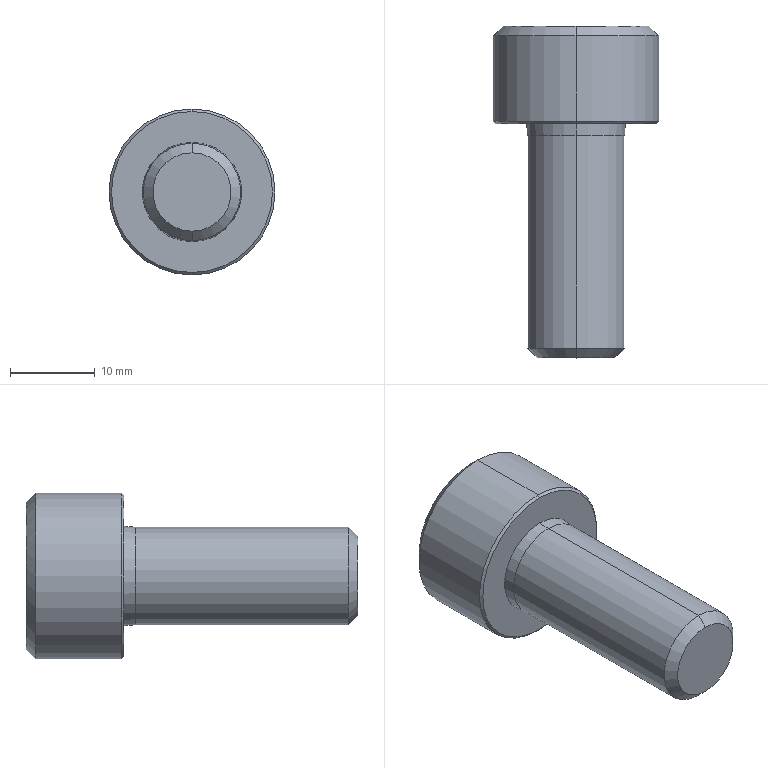Part | SolidWorks | features BaseBody 1 | 1 solid | 35 faces | box 19.615 x 39.231 x 19.615 mm | volume 5832 mm3 | cone 16 | plane 15 | cylinder 4 | commonest cylinder face diameters 11.538 x2 19.615 x2
STEP:
#1=CARTESIAN_POINT('',(-35.061,260.555,205.769));
#2=VERTEX_POINT('',#1);
#3=CARTESIAN_POINT('',(-35.061,260.555,194.231));
#4=VERTEX_POINT('',#3);
#5=CARTESIAN_POINT('',(-35.061,260.555,200.));
#6=DIRECTION('',(0.,1.,0.));
#7=DIRECTION('',(0.,0.,1.));
#8=AXIS2_PLACEMENT_3D('',#5,#6,#7);
#9=CIRCLE('',#8,5.769);
#10=EDGE_CURVE('',#2,#4,#9,.T.);
#11=ORIENTED_EDGE('',*,*,#10,.T.);
#12=CARTESIAN_POINT('',(-35.061,285.731,194.231));
#13=VERTEX_POINT('',#12);
#14=CARTESIAN_POINT('',(-35.061,259.423,194.231));
#15=DIRECTION('',(0.,1.,0.));
#16=VECTOR('',#15,1000.);
#17=LINE('',#14,#16);
#18=EDGE_CURVE('',#4,#13,#17,.T.);
#19=ORIENTED_EDGE('',*,*,#18,.T.);
#20=CARTESIAN_POINT('',(-35.061,285.731,205.769));
#21=VERTEX_POINT('',#20);
#22=CARTESIAN_POINT('',(-35.061,285.731,200.));
#23=DIRECTION('',(0.,-1.,0.));
#24=DIRECTION('',(0.,0.,1.));
#25=AXIS2_PLACEMENT_3D('',#22,#23,#24);
#26=CIRCLE('',#25,5.769);
#27=EDGE_CURVE('',#13,#21,#26,.T.);
#28=ORIENTED_EDGE('',*,*,#27,.T.);
#29=CARTESIAN_POINT('',(-35.061,259.423,205.769));
#30=DIRECTION('',(0.,1.,0.));
#31=VECTOR('',#30,1000.);
#32=LINE('',#29,#31);
#33=EDGE_CURVE('',#2,#21,#32,.T.);
#34=ORIENTED_EDGE('',*,*,#33,.F.);
#35=EDGE_LOOP('',(#11,#19,#28,#34));
#36=FACE_OUTER_BOUND('',#35,.T.);
#37=CARTESIAN_POINT('',(-35.061,259.423,200.));
#38=DIRECTION('',(0.,1.,0.));
#39=DIRECTION('',(0.,0.,1.));
#40=AXIS2_PLACEMENT_3D('',#37,#38,#39);
#41=CYLINDRICAL_SURFACE('',#40,5.769);
#42=ADVANCED_FACE('',(#36),#41,.T.);
#43=CARTESIAN_POINT('',(-35.061,259.423,204.637));
#44=VERTEX_POINT('',#43);
#45=CARTESIAN_POINT('',(-35.061,259.423,195.363));
#46=VERTEX_POINT('',#45);
#47=CARTESIAN_POINT('',(-35.061,259.423,200.));
#48=DIRECTION('',(0.,1.,0.));
#49=DIRECTION('',(0.,0.,1.));
#50=AXIS2_PLACEMENT_3D('',#47,#48,#49);
#51=CIRCLE('',#50,4.637);
#52=EDGE_CURVE('',#44,#46,#51,.T.);
#53=ORIENTED_EDGE('',*,*,#52,.T.);
#54=CARTESIAN_POINT('',(-35.061,260.555,194.231));
#55=DIRECTION('',(0.,0.7071,-0.7071));
#56=VECTOR('',#55,1000.);
#57=LINE('',#54,#56);
#58=EDGE_CURVE('',#46,#4,#57,.T.);
#59=ORIENTED_EDGE('',*,*,#58,.T.);
#60=ORIENTED_EDGE('',*,*,#10,.F.);
#61=CARTESIAN_POINT('',(-35.061,260.555,205.769));
#62=DIRECTION('',(0.,0.7071,0.7071));
#63=VECTOR('',#62,1000.);
#64=LINE('',#61,#63);
#65=EDGE_CURVE('',#44,#2,#64,.T.);
#66=ORIENTED_EDGE('',*,*,#65,.F.);
#67=EDGE_LOOP('',(#53,#59,#60,#66));
#68=FACE_OUTER_BOUND('',#67,.T.);
#69=CARTESIAN_POINT('',(-35.061,260.555,200.));
#70=DIRECTION('',(0.,1.,0.));
#71=DIRECTION('',(0.,0.,1.));
#72=AXIS2_PLACEMENT_3D('',#69,#70,#71);
#73=CONICAL_SURFACE('',#72,5.769,0.7854);
#74=ADVANCED_FACE('',(#68),#73,.T.);
#75=ORIENTED_EDGE('',*,*,#27,.F.);
#76=CARTESIAN_POINT('',(-35.061,287.115,194.115));
#77=VERTEX_POINT('',#76);
#78=CARTESIAN_POINT('',(-35.061,287.115,194.115));
#79=DIRECTION('',(0.,0.9965,-0.08305));
#80=VECTOR('',#79,1000.);
#81=LINE('',#78,#80);
#82=EDGE_CURVE('',#13,#77,#81,.T.);
#83=ORIENTED_EDGE('',*,*,#82,.T.);
#84=CARTESIAN_POINT('',(-35.061,287.115,205.885));
#85=VERTEX_POINT('',#84);
#86=CARTESIAN_POINT('',(-35.061,287.115,200.));
#87=DIRECTION('',(0.,-1.,0.));
#88=DIRECTION('',(0.,0.,1.));
#89=AXIS2_PLACEMENT_3D('',#86,#87,#88);
#90=CIRCLE('',#89,5.885);
#91=EDGE_CURVE('',#77,#85,#90,.T.);
#92=ORIENTED_EDGE('',*,*,#91,.T.);
#93=CARTESIAN_POINT('',(-35.061,287.115,205.885));
#94=DIRECTION('',(0.,0.9965,0.08305));
#95=VECTOR('',#94,1000.);
#96=LINE('',#93,#95);
#97=EDGE_CURVE('',#21,#85,#96,.T.);
#98=ORIENTED_EDGE('',*,*,#97,.F.);
#99=EDGE_LOOP('',(#75,#83,#92,#98));
#100=FACE_OUTER_BOUND('',#99,.T.);
#101=CARTESIAN_POINT('',(-35.061,287.115,200.));
#102=DIRECTION('',(0.,1.,0.));
#103=DIRECTION('',(0.,0.,1.));
#104=AXIS2_PLACEMENT_3D('',#101,#102,#103);
#105=CONICAL_SURFACE('',#104,5.885,0.08314);
#106=ADVANCED_FACE('',(#100),#105,.T.);
#107=CARTESIAN_POINT('',(-35.061,287.115,209.519));
#108=VERTEX_POINT('',#107);
#109=CARTESIAN_POINT('',(-35.061,287.115,190.481));
#110=VERTEX_POINT('',#109);
#111=CARTESIAN_POINT('',(-35.061,287.115,200.));
#112=DIRECTION('',(0.,1.,0.));
#113=DIRECTION('',(0.,0.,1.));
#114=AXIS2_PLACEMENT_3D('',#111,#112,#113);
#115=CIRCLE('',#114,9.519);
#116=EDGE_CURVE('',#108,#110,#115,.T.);
#117=ORIENTED_EDGE('',*,*,#116,.T.);
#118=CARTESIAN_POINT('',(-35.061,287.404,190.192));
#119=VERTEX_POINT('',#118);
#120=CARTESIAN_POINT('',(-35.061,287.404,190.192));
#121=DIRECTION('',(0.,0.7071,-0.7071));
#122=VECTOR('',#121,1000.);
#123=LINE('',#120,#122);
#124=EDGE_CURVE('',#110,#119,#123,.T.);
#125=ORIENTED_EDGE('',*,*,#124,.T.);
#126=CARTESIAN_POINT('',(-35.061,287.404,209.808));
#127=VERTEX_POINT('',#126);
#128=CARTESIAN_POINT('',(-35.061,287.404,200.));
#129=DIRECTION('',(0.,-1.,0.));
#130=DIRECTION('',(0.,0.,1.));
#131=AXIS2_PLACEMENT_3D('',#128,#129,#130);
#132=CIRCLE('',#131,9.808);
#133=EDGE_CURVE('',#119,#127,#132,.T.);
#134=ORIENTED_EDGE('',*,*,#133,.T.);
#135=CARTESIAN_POINT('',(-35.061,287.404,209.808));
#136=DIRECTION('',(0.,0.7071,0.7071));
#137=VECTOR('',#136,1000.);
#138=LINE('',#135,#137);
#139=EDGE_CURVE('',#108,#127,#138,.T.);
#140=ORIENTED_EDGE('',*,*,#139,.F.);
#141=EDGE_LOOP('',(#117,#125,#134,#140));
#142=FACE_OUTER_BOUND('',#141,.T.);
#143=CARTESIAN_POINT('',(-35.061,287.404,200.));
#144=DIRECTION('',(0.,1.,0.));
#145=DIRECTION('',(0.,0.,1.));
#146=AXIS2_PLACEMENT_3D('',#143,#144,#145);
#147=CONICAL_SURFACE('',#146,9.808,0.7854);
#148=ADVANCED_FACE('',(#142),#147,.T.);
#149=ORIENTED_EDGE('',*,*,#133,.F.);
#150=CARTESIAN_POINT('',(-35.061,297.5,190.192));
#151=VERTEX_POINT('',#150);
#152=CARTESIAN_POINT('',(-35.061,259.423,190.192));
#153=DIRECTION('',(0.,1.,0.));
#154=VECTOR('',#153,1000.);
#155=LINE('',#152,#154);
#156=EDGE_CURVE('',#119,#151,#155,.T.);
#157=ORIENTED_EDGE('',*,*,#156,.T.);
#158=CARTESIAN_POINT('',(-35.061,297.5,209.808));
#159=VERTEX_POINT('',#158);
#160=CARTESIAN_POINT('',(-35.061,297.5,200.));
#161=DIRECTION('',(0.,-1.,0.));
#162=DIRECTION('',(0.,0.,1.));
#163=AXIS2_PLACEMENT_3D('',#160,#161,#162);
#164=CIRCLE('',#163,9.808);
#165=EDGE_CURVE('',#151,#159,#164,.T.);
#166=ORIENTED_EDGE('',*,*,#165,.T.);
#167=CARTESIAN_POINT('',(-35.061,259.423,209.808));
#168=DIRECTION('',(0.,1.,0.));
#169=VECTOR('',#168,1000.);
#170=LINE('',#167,#169);
#171=EDGE_CURVE('',#127,#159,#170,.T.);
#172=ORIENTED_EDGE('',*,*,#171,.F.);
#173=EDGE_LOOP('',(#149,#157,#166,#172));
#174=FACE_OUTER_BOUND('',#173,.T.);
#175=CARTESIAN_POINT('',(-35.061,259.423,200.));
#176=DIRECTION('',(0.,1.,0.));
#177=DIRECTION('',(0.,0.,1.));
#178=AXIS2_PLACEMENT_3D('',#175,#176,#177);
#179=CYLINDRICAL_SURFACE('',#178,9.808);
#180=ADVANCED_FACE('',(#174),#179,.T.);
#181=CARTESIAN_POINT('',(-35.061,298.654,191.346));
#182=VERTEX_POINT('',#181);
#183=CARTESIAN_POINT('',(-35.061,298.654,208.654));
#184=VERTEX_POINT('',#183);
#185=CARTESIAN_POINT('',(-35.061,298.654,200.));
#186=DIRECTION('',(0.,-1.,0.));
#187=DIRECTION('',(0.,0.,-1.));
#188=AXIS2_PLACEMENT_3D('',#185,#186,#187);
#189=CIRCLE('',#188,8.654);
#190=EDGE_CURVE('',#182,#184,#189,.T.);
#191=ORIENTED_EDGE('',*,*,#190,.T.);
#192=CARTESIAN_POINT('',(-35.061,297.5,209.808));
#193=DIRECTION('',(0.,-0.7071,0.7071));
#194=VECTOR('',#193,1000.);
#195=LINE('',#192,#194);
#196=EDGE_CURVE('',#184,#159,#195,.T.);
#197=ORIENTED_EDGE('',*,*,#196,.T.);
#198=ORIENTED_EDGE('',*,*,#165,.F.);
#199=CARTESIAN_POINT('',(-35.061,297.5,190.192));
#200=DIRECTION('',(0.,-0.7071,-0.7071));
#201=VECTOR('',#200,1000.);
#202=LINE('',#199,#201);
#203=EDGE_CURVE('',#182,#151,#202,.T.);
#204=ORIENTED_EDGE('',*,*,#203,.F.);
#205=EDGE_LOOP('',(#191,#197,#198,#204));
#206=FACE_OUTER_BOUND('',#205,.T.);
#207=CARTESIAN_POINT('',(-35.061,297.5,200.));
#208=DIRECTION('',(0.,-1.,0.));
#209=DIRECTION('',(0.,0.,-1.));
#210=AXIS2_PLACEMENT_3D('',#207,#208,#209);
#211=CONICAL_SURFACE('',#210,9.808,0.7854);
#212=ADVANCED_FACE('',(#206),#211,.T.);
#213=CARTESIAN_POINT('',(-35.061,290.22,200.));
#214=VERTEX_POINT('',#213);
#215=CARTESIAN_POINT('',(-35.061,292.885,204.615));
#216=VERTEX_POINT('',#215);
#217=CARTESIAN_POINT('',(-35.061,292.885,204.615));
#218=DIRECTION('',(0.,0.5,0.866));
#219=VECTOR('',#218,1000.);
#220=LINE('',#217,#219);
#221=EDGE_CURVE('',#214,#216,#220,.T.);
#222=ORIENTED_EDGE('',*,*,#221,.F.);
#223=CARTESIAN_POINT('',(-35.061,292.885,195.385));
#224=VERTEX_POINT('',#223);
#225=CARTESIAN_POINT('',(-35.061,292.885,195.385));
#226=DIRECTION('',(0.,0.5,-0.866));
#227=VECTOR('',#226,1000.);
#228=LINE('',#225,#227);
#229=EDGE_CURVE('',#214,#224,#228,.T.);
#230=ORIENTED_EDGE('',*,*,#229,.T.);
#231=CARTESIAN_POINT('',(-37.369,292.885,196.003));
#232=VERTEX_POINT('',#231);
#233=CARTESIAN_POINT('',(-35.061,292.885,200.));
#234=DIRECTION('',(0.,-1.,0.));
#235=DIRECTION('',(0.,0.,1.));
#236=AXIS2_PLACEMENT_3D('',#233,#234,#235);
#237=CIRCLE('',#236,4.615);
#238=EDGE_CURVE('',#232,#224,#237,.T.);
#239=ORIENTED_EDGE('',*,*,#238,.F.);
#240=CARTESIAN_POINT('',(-39.677,292.885,200.));
#241=VERTEX_POINT('',#240);
#242=CARTESIAN_POINT('',(-35.061,292.885,200.));
#243=DIRECTION('',(0.,-1.,0.));
#244=DIRECTION('',(0.,0.,1.));
#245=AXIS2_PLACEMENT_3D('',#242,#243,#244);
#246=CIRCLE('',#245,4.615);
#247=EDGE_CURVE('',#241,#232,#246,.T.);
#248=ORIENTED_EDGE('',*,*,#247,.F.);
#249=CARTESIAN_POINT('',(-37.369,292.885,203.997));
#250=VERTEX_POINT('',#249);
#251=CARTESIAN_POINT('',(-35.061,292.885,200.));
#252=DIRECTION('',(0.,-1.,0.));
#253=DIRECTION('',(0.,0.,1.));
#254=AXIS2_PLACEMENT_3D('',#251,#252,#253);
#255=CIRCLE('',#254,4.615);
#256=EDGE_CURVE('',#250,#241,#255,.T.);
#257=ORIENTED_EDGE('',*,*,#256,.F.);
#258=CARTESIAN_POINT('',(-35.061,292.885,200.));
#259=DIRECTION('',(0.,-1.,0.));
#260=DIRECTION('',(0.,0.,1.));
#261=AXIS2_PLACEMENT_3D('',#258,#259,#260);
#262=CIRCLE('',#261,4.615);
#263=EDGE_CURVE('',#216,#250,#262,.T.);
#264=ORIENTED_EDGE('',*,*,#263,.F.);
#265=EDGE_LOOP('',(#222,#230,#239,#248,#257,#264));
#266=FACE_OUTER_BOUND('',#265,.T.);
#267=CARTESIAN_POINT('',(-35.061,292.885,200.));
#268=DIRECTION('',(0.,1.,0.));
#269=DIRECTION('',(0.,0.,1.));
#270=AXIS2_PLACEMENT_3D('',#267,#268,#269);
#271=CONICAL_SURFACE('',#270,4.615,1.047);
#272=ADVANCED_FACE('',(#266),#271,.F.);
#273=ORIENTED_EDGE('',*,*,#18,.F.);
#274=CARTESIAN_POINT('',(-35.061,260.555,200.));
#275=DIRECTION('',(0.,1.,0.));
#276=DIRECTION('',(0.,0.,1.));
#277=AXIS2_PLACEMENT_3D('',#274,#275,#276);
#278=CIRCLE('',#277,5.769);
#279=EDGE_CURVE('',#4,#2,#278,.T.);
#280=ORIENTED_EDGE('',*,*,#279,.T.);
#281=ORIENTED_EDGE('',*,*,#33,.T.);
#282=CARTESIAN_POINT('',(-35.061,285.731,200.));
#283=DIRECTION('',(0.,-1.,0.));
#284=DIRECTION('',(0.,0.,1.));
#285=AXIS2_PLACEMENT_3D('',#282,#283,#284);
#286=CIRCLE('',#285,5.769);
#287=EDGE_CURVE('',#21,#13,#286,.T.);
#288=ORIENTED_EDGE('',*,*,#287,.T.);
#289=EDGE_LOOP('',(#273,#280,#281,#288));
#290=FACE_OUTER_BOUND('',#289,.T.);
#291=CARTESIAN_POINT('',(-35.061,259.423,200.));
#292=DIRECTION('',(0.,1.,0.));
#293=DIRECTION('',(0.,0.,1.));
#294=AXIS2_PLACEMENT_3D('',#291,#292,#293);
#295=CYLINDRICAL_SURFACE('',#294,5.769);
#296=ADVANCED_FACE('',(#290),#295,.T.);
#297=ORIENTED_EDGE('',*,*,#58,.F.);
#298=CARTESIAN_POINT('',(-35.061,259.423,200.));
#299=DIRECTION('',(0.,1.,0.));
#300=DIRECTION('',(0.,0.,1.));
#301=AXIS2_PLACEMENT_3D('',#298,#299,#300);
#302=CIRCLE('',#301,4.637);
#303=EDGE_CURVE('',#46,#44,#302,.T.);
#304=ORIENTED_EDGE('',*,*,#303,.T.);
#305=ORIENTED_EDGE('',*,*,#65,.T.);
#306=ORIENTED_EDGE('',*,*,#279,.F.);
#307=EDGE_LOOP('',(#297,#304,#305,#306));
#308=FACE_OUTER_BOUND('',#307,.T.);
#309=CARTESIAN_POINT('',(-35.061,260.555,200.));
#310=DIRECTION('',(0.,1.,0.));
#311=DIRECTION('',(0.,0.,1.));
#312=AXIS2_PLACEMENT_3D('',#309,#310,#311);
#313=CONICAL_SURFACE('',#312,5.769,0.7854);
#314=ADVANCED_FACE('',(#308),#313,.T.);
#315=ORIENTED_EDGE('',*,*,#82,.F.);
#316=ORIENTED_EDGE('',*,*,#287,.F.);
#317=ORIENTED_EDGE('',*,*,#97,.T.);
#318=CARTESIAN_POINT('',(-35.061,287.115,200.));
#319=DIRECTION('',(0.,-1.,0.));
#320=DIRECTION('',(0.,0.,1.));
#321=AXIS2_PLACEMENT_3D('',#318,#319,#320);
#322=CIRCLE('',#321,5.885);
#323=EDGE_CURVE('',#85,#77,#322,.T.);
#324=ORIENTED_EDGE('',*,*,#323,.T.);
#325=EDGE_LOOP('',(#315,#316,#317,#324));
#326=FACE_OUTER_BOUND('',#325,.T.);
#327=CARTESIAN_POINT('',(-35.061,287.115,200.));
#328=DIRECTION('',(0.,1.,0.));
#329=DIRECTION('',(0.,0.,1.));
#330=AXIS2_PLACEMENT_3D('',#327,#328,#329);
#331=CONICAL_SURFACE('',#330,5.885,0.08314);
#332=ADVANCED_FACE('',(#326),#331,.T.);
#333=ORIENTED_EDGE('',*,*,#52,.F.);
#334=ORIENTED_EDGE('',*,*,#303,.F.);
#335=EDGE_LOOP('',(#333,#334));
#336=FACE_OUTER_BOUND('',#335,.T.);
#337=CARTESIAN_POINT('',(-39.698,259.423,200.));
#338=DIRECTION('',(0.,1.,0.));
#339=DIRECTION('',(0.,0.,1.));
#340=AXIS2_PLACEMENT_3D('',#337,#338,#339);
#341=PLANE('',#340);
#342=ADVANCED_FACE('',(#336),#341,.F.);
#343=ORIENTED_EDGE('',*,*,#323,.F.);
#344=ORIENTED_EDGE('',*,*,#91,.F.);
#345=EDGE_LOOP('',(#343,#344));
#346=FACE_BOUND('',#345,.T.);
#347=ORIENTED_EDGE('',*,*,#116,.F.);
#348=CARTESIAN_POINT('',(-35.061,287.115,200.));
#349=DIRECTION('',(0.,1.,0.));
#350=DIRECTION('',(0.,0.,1.));
#351=AXIS2_PLACEMENT_3D('',#348,#349,#350);
#352=CIRCLE('',#351,9.519);
#353=EDGE_CURVE('',#110,#108,#352,.T.);
#354=ORIENTED_EDGE('',*,*,#353,.F.);
#355=EDGE_LOOP('',(#347,#354));
#356=FACE_OUTER_BOUND('',#355,.T.);
#357=CARTESIAN_POINT('',(-44.58,287.115,200.));
#358=DIRECTION('',(0.,1.,0.));
#359=DIRECTION('',(0.,0.,1.));
#360=AXIS2_PLACEMENT_3D('',#357,#358,#359);
#361=PLANE('',#360);
#362=ADVANCED_FACE('',(#346,#356),#361,.F.);
#363=ORIENTED_EDGE('',*,*,#124,.F.);
#364=ORIENTED_EDGE('',*,*,#353,.T.);
#365=ORIENTED_EDGE('',*,*,#139,.T.);
#366=CARTESIAN_POINT('',(-35.061,287.404,200.));
#367=DIRECTION('',(0.,-1.,0.));
#368=DIRECTION('',(0.,0.,1.));
#369=AXIS2_PLACEMENT_3D('',#366,#367,#368);
#370=CIRCLE('',#369,9.808);
#371=EDGE_CURVE('',#127,#119,#370,.T.);
#372=ORIENTED_EDGE('',*,*,#371,.T.);
#373=EDGE_LOOP('',(#363,#364,#365,#372));
#374=FACE_OUTER_BOUND('',#373,.T.);
#375=CARTESIAN_POINT('',(-35.061,287.404,200.));
#376=DIRECTION('',(0.,1.,0.));
#377=DIRECTION('',(0.,0.,1.));
#378=AXIS2_PLACEMENT_3D('',#375,#376,#377);
#379=CONICAL_SURFACE('',#378,9.808,0.7854);
#380=ADVANCED_FACE('',(#374),#379,.T.);
#381=ORIENTED_EDGE('',*,*,#156,.F.);
#382=ORIENTED_EDGE('',*,*,#371,.F.);
#383=ORIENTED_EDGE('',*,*,#171,.T.);
#384=CARTESIAN_POINT('',(-35.061,297.5,200.));
#385=DIRECTION('',(0.,-1.,0.));
#386=DIRECTION('',(0.,0.,1.));
#387=AXIS2_PLACEMENT_3D('',#384,#385,#386);
#388=CIRCLE('',#387,9.808);
#389=EDGE_CURVE('',#159,#151,#388,.T.);
#390=ORIENTED_EDGE('',*,*,#389,.T.);
#391=EDGE_LOOP('',(#381,#382,#383,#390));
#392=FACE_OUTER_BOUND('',#391,.T.);
#393=CARTESIAN_POINT('',(-35.061,259.423,200.));
#394=DIRECTION('',(0.,1.,0.));
#395=DIRECTION('',(0.,0.,1.));
#396=AXIS2_PLACEMENT_3D('',#393,#394,#395);
#397=CYLINDRICAL_SURFACE('',#396,9.808);
#398=ADVANCED_FACE('',(#392),#397,.T.);
#399=ORIENTED_EDGE('',*,*,#196,.F.);
#400=CARTESIAN_POINT('',(-35.061,298.654,200.));
#401=DIRECTION('',(0.,-1.,0.));
#402=DIRECTION('',(0.,0.,-1.));
#403=AXIS2_PLACEMENT_3D('',#400,#401,#402);
#404=CIRCLE('',#403,8.654);
#405=EDGE_CURVE('',#184,#182,#404,.T.);
#406=ORIENTED_EDGE('',*,*,#405,.T.);
#407=ORIENTED_EDGE('',*,*,#203,.T.);
#408=ORIENTED_EDGE('',*,*,#389,.F.);
#409=EDGE_LOOP('',(#399,#406,#407,#408));
#410=FACE_OUTER_BOUND('',#409,.T.);
#411=CARTESIAN_POINT('',(-35.061,297.5,200.));
#412=DIRECTION('',(0.,-1.,0.));
#413=DIRECTION('',(0.,0.,-1.));
#414=AXIS2_PLACEMENT_3D('',#411,#412,#413);
#415=CONICAL_SURFACE('',#414,9.808,0.7854);
#416=ADVANCED_FACE('',(#410),#415,.T.);
#417=CARTESIAN_POINT('',(-30.446,298.654,197.335));
#418=VERTEX_POINT('',#417);
#419=CARTESIAN_POINT('',(-35.061,298.654,194.671));
#420=VERTEX_POINT('',#419);
#421=CARTESIAN_POINT('',(-35.061,298.654,200.));
#422=DIRECTION('',(0.,1.,0.));
#423=DIRECTION('',(0.,0.,1.));
#424=AXIS2_PLACEMENT_3D('',#421,#422,#423);
#425=CIRCLE('',#424,5.329);
#426=EDGE_CURVE('',#418,#420,#425,.T.);
#427=ORIENTED_EDGE('',*,*,#426,.F.);
#428=CARTESIAN_POINT('',(-30.446,298.654,202.665));
#429=VERTEX_POINT('',#428);
#430=CARTESIAN_POINT('',(-35.061,298.654,200.));
#431=DIRECTION('',(0.,1.,0.));
#432=DIRECTION('',(0.,0.,1.));
#433=AXIS2_PLACEMENT_3D('',#430,#431,#432);
#434=CIRCLE('',#433,5.329);
#435=EDGE_CURVE('',#429,#418,#434,.T.);
#436=ORIENTED_EDGE('',*,*,#435,.F.);
#437=CARTESIAN_POINT('',(-35.061,298.654,205.329));
#438=VERTEX_POINT('',#437);
#439=CARTESIAN_POINT('',(-35.061,298.654,200.));
#440=DIRECTION('',(0.,1.,0.));
#441=DIRECTION('',(0.,0.,1.));
#442=AXIS2_PLACEMENT_3D('',#439,#440,#441);
#443=CIRCLE('',#442,5.329);
#444=EDGE_CURVE('',#438,#429,#443,.T.);
#445=ORIENTED_EDGE('',*,*,#444,.F.);
#446=CARTESIAN_POINT('',(-39.677,298.654,202.665));
#447=VERTEX_POINT('',#446);
#448=CARTESIAN_POINT('',(-35.061,298.654,200.));
#449=DIRECTION('',(0.,1.,0.));
#450=DIRECTION('',(0.,0.,1.));
#451=AXIS2_PLACEMENT_3D('',#448,#449,#450);
#452=CIRCLE('',#451,5.329);
#453=EDGE_CURVE('',#447,#438,#452,.T.);
#454=ORIENTED_EDGE('',*,*,#453,.F.);
#455=CARTESIAN_POINT('',(-39.677,298.654,197.335));
#456=VERTEX_POINT('',#455);
#457=CARTESIAN_POINT('',(-35.061,298.654,200.));
#458=DIRECTION('',(0.,1.,0.));
#459=DIRECTION('',(0.,0.,1.));
#460=AXIS2_PLACEMENT_3D('',#457,#458,#459);
#461=CIRCLE('',#460,5.329);
#462=EDGE_CURVE('',#456,#447,#461,.T.);
#463=ORIENTED_EDGE('',*,*,#462,.F.);
#464=CARTESIAN_POINT('',(-35.061,298.654,200.));
#465=DIRECTION('',(0.,1.,0.));
#466=DIRECTION('',(0.,0.,1.));
#467=AXIS2_PLACEMENT_3D('',#464,#465,#466);
#468=CIRCLE('',#467,5.329);
#469=EDGE_CURVE('',#420,#456,#468,.T.);
#470=ORIENTED_EDGE('',*,*,#469,.F.);
#471=EDGE_LOOP('',(#427,#436,#445,#454,#463,#470));
#472=FACE_BOUND('',#471,.T.);
#473=ORIENTED_EDGE('',*,*,#190,.F.);
#474=ORIENTED_EDGE('',*,*,#405,.F.);
#475=EDGE_LOOP('',(#473,#474));
#476=FACE_OUTER_BOUND('',#475,.T.);
#477=CARTESIAN_POINT('',(-40.391,298.654,200.));
#478=DIRECTION('',(0.,-1.,0.));
#479=DIRECTION('',(0.,0.,-1.));
#480=AXIS2_PLACEMENT_3D('',#477,#478,#479);
#481=PLANE('',#480);
#482=ADVANCED_FACE('',(#472,#476),#481,.F.);
#483=CARTESIAN_POINT('',(-35.061,298.654,194.671));
#484=CARTESIAN_POINT('',(-35.422,298.446,194.879));
#485=CARTESIAN_POINT('',(-35.791,298.269,195.092));
#486=CARTESIAN_POINT('',(-36.363,298.079,195.422));
#487=CARTESIAN_POINT('',(-36.558,298.029,195.535));
#488=CARTESIAN_POINT('',(-36.955,297.959,195.764));
#489=CARTESIAN_POINT('',(-37.159,297.94,195.882));
#490=CARTESIAN_POINT('',(-37.763,297.939,196.231));
#491=CARTESIAN_POINT('',(-38.159,298.009,196.459));
#492=CARTESIAN_POINT('',(-38.94,298.265,196.91));
#493=CARTESIAN_POINT('',(-39.314,298.444,197.126));
#494=CARTESIAN_POINT('',(-39.677,298.654,197.335));
#495=B_SPLINE_CURVE_WITH_KNOTS('',3,(#483,#484,#485,#486,#487,#488,#489,#490,#491,#492,#493,#494),.UNSPECIFIED.,.F.,.F.,(4,2,2,2,2,4),(0.,0.001376,0.002064,0.002753,0.004129,0.005505),.UNSPECIFIED.);
#496=EDGE_CURVE('',#420,#456,#495,.T.);
#497=ORIENTED_EDGE('',*,*,#496,.F.);
#498=ORIENTED_EDGE('',*,*,#469,.T.);
#499=EDGE_LOOP('',(#497,#498));
#500=FACE_OUTER_BOUND('',#499,.T.);
#501=CARTESIAN_POINT('',(-35.061,298.654,200.));
#502=DIRECTION('',(0.,1.,0.));
#503=DIRECTION('',(0.,0.,1.));
#504=AXIS2_PLACEMENT_3D('',#501,#502,#503);
#505=CONICAL_SURFACE('',#504,5.329,0.7854);
#506=ADVANCED_FACE('',(#500),#505,.F.);
#507=CARTESIAN_POINT('',(-30.446,298.654,197.335));
#508=CARTESIAN_POINT('',(-30.806,298.446,197.127));
#509=CARTESIAN_POINT('',(-31.175,298.269,196.914));
#510=CARTESIAN_POINT('',(-31.748,298.079,196.583));
#511=CARTESIAN_POINT('',(-31.942,298.029,196.471));
#512=CARTESIAN_POINT('',(-32.339,297.959,196.242));
#513=CARTESIAN_POINT('',(-32.544,297.94,196.124));
#514=CARTESIAN_POINT('',(-33.148,297.939,195.775));
#515=CARTESIAN_POINT('',(-33.544,298.009,195.547));
#516=CARTESIAN_POINT('',(-34.325,298.265,195.096));
#517=CARTESIAN_POINT('',(-34.698,298.444,194.88));
#518=CARTESIAN_POINT('',(-35.061,298.654,194.671));
#519=B_SPLINE_CURVE_WITH_KNOTS('',3,(#507,#508,#509,#510,#511,#512,#513,#514,#515,#516,#517,#518),.UNSPECIFIED.,.F.,.F.,(4,2,2,2,2,4),(0.,0.001376,0.002064,0.002753,0.004129,0.005505),.UNSPECIFIED.);
#520=EDGE_CURVE('',#418,#420,#519,.T.);
#521=ORIENTED_EDGE('',*,*,#520,.F.);
#522=ORIENTED_EDGE('',*,*,#426,.T.);
#523=EDGE_LOOP('',(#521,#522));
#524=FACE_OUTER_BOUND('',#523,.T.);
#525=CARTESIAN_POINT('',(-35.061,298.654,200.));
#526=DIRECTION('',(0.,1.,0.));
#527=DIRECTION('',(0.,0.,1.));
#528=AXIS2_PLACEMENT_3D('',#525,#526,#527);
#529=CONICAL_SURFACE('',#528,5.329,0.7854);
#530=ADVANCED_FACE('',(#524),#529,.F.);
#531=CARTESIAN_POINT('',(-30.446,298.654,202.665));
#532=CARTESIAN_POINT('',(-30.446,298.446,202.248));
#533=CARTESIAN_POINT('',(-30.446,298.269,201.823));
#534=CARTESIAN_POINT('',(-30.446,298.079,201.161));
#535=CARTESIAN_POINT('',(-30.446,298.029,200.937));
#536=CARTESIAN_POINT('',(-30.446,297.959,200.478));
#537=CARTESIAN_POINT('',(-30.446,297.94,200.242));
#538=CARTESIAN_POINT('',(-30.446,297.939,199.545));
#539=CARTESIAN_POINT('',(-30.446,298.009,199.087));
#540=CARTESIAN_POINT('',(-30.446,298.265,198.185));
#541=CARTESIAN_POINT('',(-30.446,298.444,197.754));
#542=CARTESIAN_POINT('',(-30.446,298.654,197.335));
#543=B_SPLINE_CURVE_WITH_KNOTS('',3,(#531,#532,#533,#534,#535,#536,#537,#538,#539,#540,#541,#542),.UNSPECIFIED.,.F.,.F.,(4,2,2,2,2,4),(0.,0.001376,0.002064,0.002753,0.004129,0.005505),.UNSPECIFIED.);
#544=EDGE_CURVE('',#429,#418,#543,.T.);
#545=ORIENTED_EDGE('',*,*,#544,.F.);
#546=ORIENTED_EDGE('',*,*,#435,.T.);
#547=EDGE_LOOP('',(#545,#546));
#548=FACE_OUTER_BOUND('',#547,.T.);
#549=CARTESIAN_POINT('',(-35.061,298.654,200.));
#550=DIRECTION('',(0.,1.,0.));
#551=DIRECTION('',(0.,0.,1.));
#552=AXIS2_PLACEMENT_3D('',#549,#550,#551);
#553=CONICAL_SURFACE('',#552,5.329,0.7854);
#554=ADVANCED_FACE('',(#548),#553,.F.);
#555=CARTESIAN_POINT('',(-35.061,298.654,205.329));
#556=CARTESIAN_POINT('',(-34.701,298.446,205.121));
#557=CARTESIAN_POINT('',(-34.332,298.269,204.908));
#558=CARTESIAN_POINT('',(-33.759,298.079,204.578));
#559=CARTESIAN_POINT('',(-33.565,298.029,204.465));
#560=CARTESIAN_POINT('',(-33.168,297.959,204.236));
#561=CARTESIAN_POINT('',(-32.963,297.94,204.118));
#562=CARTESIAN_POINT('',(-32.359,297.939,203.769));
#563=CARTESIAN_POINT('',(-31.963,298.009,203.541));
#564=CARTESIAN_POINT('',(-31.182,298.265,203.09));
#565=CARTESIAN_POINT('',(-30.809,298.444,202.874));
#566=CARTESIAN_POINT('',(-30.446,298.654,202.665));
#567=B_SPLINE_CURVE_WITH_KNOTS('',3,(#555,#556,#557,#558,#559,#560,#561,#562,#563,#564,#565,#566),.UNSPECIFIED.,.F.,.F.,(4,2,2,2,2,4),(0.,0.001376,0.002064,0.002753,0.004129,0.005505),.UNSPECIFIED.);
#568=EDGE_CURVE('',#438,#429,#567,.T.);
#569=ORIENTED_EDGE('',*,*,#568,.F.);
#570=ORIENTED_EDGE('',*,*,#444,.T.);
#571=EDGE_LOOP('',(#569,#570));
#572=FACE_OUTER_BOUND('',#571,.T.);
#573=CARTESIAN_POINT('',(-35.061,298.654,200.));
#574=DIRECTION('',(0.,1.,0.));
#575=DIRECTION('',(0.,0.,1.));
#576=AXIS2_PLACEMENT_3D('',#573,#574,#575);
#577=CONICAL_SURFACE('',#576,5.329,0.7854);
#578=ADVANCED_FACE('',(#572),#577,.F.);
#579=CARTESIAN_POINT('',(-39.677,298.654,202.665));
#580=CARTESIAN_POINT('',(-39.316,298.446,202.873));
#581=CARTESIAN_POINT('',(-38.947,298.269,203.086));
#582=CARTESIAN_POINT('',(-38.374,298.079,203.417));
#583=CARTESIAN_POINT('',(-38.18,298.029,203.529));
#584=CARTESIAN_POINT('',(-37.783,297.959,203.758));
#585=CARTESIAN_POINT('',(-37.579,297.94,203.876));
#586=CARTESIAN_POINT('',(-36.974,297.939,204.225));
#587=CARTESIAN_POINT('',(-36.578,298.009,204.453));
#588=CARTESIAN_POINT('',(-35.797,298.265,204.904));
#589=CARTESIAN_POINT('',(-35.424,298.444,205.12));
#590=CARTESIAN_POINT('',(-35.061,298.654,205.329));
#591=B_SPLINE_CURVE_WITH_KNOTS('',3,(#579,#580,#581,#582,#583,#584,#585,#586,#587,#588,#589,#590),.UNSPECIFIED.,.F.,.F.,(4,2,2,2,2,4),(0.,0.001376,0.002064,0.002753,0.004129,0.005505),.UNSPECIFIED.);
#592=EDGE_CURVE('',#447,#438,#591,.T.);
#593=ORIENTED_EDGE('',*,*,#592,.F.);
#594=ORIENTED_EDGE('',*,*,#453,.T.);
#595=EDGE_LOOP('',(#593,#594));
#596=FACE_OUTER_BOUND('',#595,.T.);
#597=CARTESIAN_POINT('',(-35.061,298.654,200.));
#598=DIRECTION('',(0.,1.,0.));
#599=DIRECTION('',(0.,0.,1.));
#600=AXIS2_PLACEMENT_3D('',#597,#598,#599);
#601=CONICAL_SURFACE('',#600,5.329,0.7854);
#602=ADVANCED_FACE('',(#596),#601,.F.);
#603=CARTESIAN_POINT('',(-39.677,298.654,197.335));
#604=CARTESIAN_POINT('',(-39.677,298.446,197.752));
#605=CARTESIAN_POINT('',(-39.677,298.269,198.177));
#606=CARTESIAN_POINT('',(-39.677,298.079,198.839));
#607=CARTESIAN_POINT('',(-39.677,298.029,199.063));
#608=CARTESIAN_POINT('',(-39.677,297.959,199.522));
#609=CARTESIAN_POINT('',(-39.677,297.94,199.758));
#610=CARTESIAN_POINT('',(-39.677,297.939,200.455));
#611=CARTESIAN_POINT('',(-39.677,298.009,200.913));
#612=CARTESIAN_POINT('',(-39.677,298.265,201.815));
#613=CARTESIAN_POINT('',(-39.677,298.444,202.246));
#614=CARTESIAN_POINT('',(-39.677,298.654,202.665));
#615=B_SPLINE_CURVE_WITH_KNOTS('',3,(#603,#604,#605,#606,#607,#608,#609,#610,#611,#612,#613,#614),.UNSPECIFIED.,.F.,.F.,(4,2,2,2,2,4),(0.,0.001376,0.002064,0.002753,0.004129,0.005505),.UNSPECIFIED.);
#616=EDGE_CURVE('',#456,#447,#615,.T.);
#617=ORIENTED_EDGE('',*,*,#616,.F.);
#618=ORIENTED_EDGE('',*,*,#462,.T.);
#619=EDGE_LOOP('',(#617,#618));
#620=FACE_OUTER_BOUND('',#619,.T.);
#621=CARTESIAN_POINT('',(-35.061,298.654,200.));
#622=DIRECTION('',(0.,1.,0.));
#623=DIRECTION('',(0.,0.,1.));
#624=AXIS2_PLACEMENT_3D('',#621,#622,#623);
#625=CONICAL_SURFACE('',#624,5.329,0.7854);
#626=ADVANCED_FACE('',(#620),#625,.F.);
#627=CARTESIAN_POINT('',(-39.677,292.885,197.335));
#628=VERTEX_POINT('',#627);
#629=CARTESIAN_POINT('',(-39.677,292.885,197.335));
#630=DIRECTION('',(0.,1.,0.));
#631=VECTOR('',#630,1000.);
#632=LINE('',#629,#631);
#633=EDGE_CURVE('',#628,#456,#632,.T.);
#634=ORIENTED_EDGE('',*,*,#633,.F.);
#635=CARTESIAN_POINT('',(-35.061,292.885,194.671));
#636=DIRECTION('',(-0.866,0.,0.5));
#637=VECTOR('',#636,1000.);
#638=LINE('',#635,#637);
#639=EDGE_CURVE('',#232,#628,#638,.T.);
#640=ORIENTED_EDGE('',*,*,#639,.F.);
#641=CARTESIAN_POINT('',(-35.061,292.885,194.671));
#642=VERTEX_POINT('',#641);
#643=CARTESIAN_POINT('',(-35.061,292.885,194.671));
#644=DIRECTION('',(-0.866,0.,0.5));
#645=VECTOR('',#644,1000.);
#646=LINE('',#643,#645);
#647=EDGE_CURVE('',#642,#232,#646,.T.);
#648=ORIENTED_EDGE('',*,*,#647,.F.);
#649=CARTESIAN_POINT('',(-35.061,292.885,194.671));
#650=DIRECTION('',(0.,-1.,0.));
#651=VECTOR('',#650,1000.);
#652=LINE('',#649,#651);
#653=EDGE_CURVE('',#420,#642,#652,.T.);
#654=ORIENTED_EDGE('',*,*,#653,.F.);
#655=ORIENTED_EDGE('',*,*,#496,.T.);
#656=EDGE_LOOP('',(#634,#640,#648,#654,#655));
#657=FACE_OUTER_BOUND('',#656,.T.);
#658=CARTESIAN_POINT('',(-35.061,292.885,194.671));
#659=DIRECTION('',(-0.5,0.,-0.866));
#660=DIRECTION('',(-0.866,0.,0.5));
#661=AXIS2_PLACEMENT_3D('',#658,#659,#660);
#662=PLANE('',#661);
#663=ADVANCED_FACE('',(#657),#662,.F.);
#664=ORIENTED_EDGE('',*,*,#653,.T.);
#665=CARTESIAN_POINT('',(-32.753,292.885,196.003));
#666=VERTEX_POINT('',#665);
#667=CARTESIAN_POINT('',(-30.446,292.885,197.335));
#668=DIRECTION('',(-0.866,0.,-0.5));
#669=VECTOR('',#668,1000.);
#670=LINE('',#667,#669);
#671=EDGE_CURVE('',#666,#642,#670,.T.);
#672=ORIENTED_EDGE('',*,*,#671,.F.);
#673=CARTESIAN_POINT('',(-30.446,292.885,197.335));
#674=VERTEX_POINT('',#673);
#675=CARTESIAN_POINT('',(-30.446,292.885,197.335));
#676=DIRECTION('',(-0.866,0.,-0.5));
#677=VECTOR('',#676,1000.);
#678=LINE('',#675,#677);
#679=EDGE_CURVE('',#674,#666,#678,.T.);
#680=ORIENTED_EDGE('',*,*,#679,.F.);
#681=CARTESIAN_POINT('',(-30.446,292.885,197.335));
#682=DIRECTION('',(0.,-1.,0.));
#683=VECTOR('',#682,1000.);
#684=LINE('',#681,#683);
#685=EDGE_CURVE('',#418,#674,#684,.T.);
#686=ORIENTED_EDGE('',*,*,#685,.F.);
#687=ORIENTED_EDGE('',*,*,#520,.T.);
#688=EDGE_LOOP('',(#664,#672,#680,#686,#687));
#689=FACE_OUTER_BOUND('',#688,.T.);
#690=CARTESIAN_POINT('',(-30.446,292.885,197.335));
#691=DIRECTION('',(0.5,0.,-0.866));
#692=DIRECTION('',(-0.866,0.,-0.5));
#693=AXIS2_PLACEMENT_3D('',#690,#691,#692);
#694=PLANE('',#693);
#695=ADVANCED_FACE('',(#689),#694,.F.);
#696=ORIENTED_EDGE('',*,*,#685,.T.);
#697=CARTESIAN_POINT('',(-30.446,292.885,200.));
#698=VERTEX_POINT('',#697);
#699=CARTESIAN_POINT('',(-30.446,292.885,202.665));
#700=DIRECTION('',(0.,0.,-1.));
#701=VECTOR('',#700,1000.);
#702=LINE('',#699,#701);
#703=EDGE_CURVE('',#698,#674,#702,.T.);
#704=ORIENTED_EDGE('',*,*,#703,.F.);
#705=CARTESIAN_POINT('',(-30.446,292.885,202.665));
#706=VERTEX_POINT('',#705);
#707=CARTESIAN_POINT('',(-30.446,292.885,202.665));
#708=DIRECTION('',(0.,0.,-1.));
#709=VECTOR('',#708,1000.);
#710=LINE('',#707,#709);
#711=EDGE_CURVE('',#706,#698,#710,.T.);
#712=ORIENTED_EDGE('',*,*,#711,.F.);
#713=CARTESIAN_POINT('',(-30.446,292.885,202.665));
#714=DIRECTION('',(0.,-1.,0.));
#715=VECTOR('',#714,1000.);
#716=LINE('',#713,#715);
#717=EDGE_CURVE('',#429,#706,#716,.T.);
#718=ORIENTED_EDGE('',*,*,#717,.F.);
#719=ORIENTED_EDGE('',*,*,#544,.T.);
#720=EDGE_LOOP('',(#696,#704,#712,#718,#719));
#721=FACE_OUTER_BOUND('',#720,.T.);
#722=CARTESIAN_POINT('',(-30.446,292.885,202.665));
#723=DIRECTION('',(1.,0.,0.));
#724=DIRECTION('',(0.,0.,-1.));
#725=AXIS2_PLACEMENT_3D('',#722,#723,#724);
#726=PLANE('',#725);
#727=ADVANCED_FACE('',(#721),#726,.F.);
#728=ORIENTED_EDGE('',*,*,#717,.T.);
#729=CARTESIAN_POINT('',(-32.753,292.885,203.997));
#730=VERTEX_POINT('',#729);
#731=CARTESIAN_POINT('',(-35.061,292.885,205.329));
#732=DIRECTION('',(0.866,0.,-0.5));
#733=VECTOR('',#732,1000.);
#734=LINE('',#731,#733);
#735=EDGE_CURVE('',#730,#706,#734,.T.);
#736=ORIENTED_EDGE('',*,*,#735,.F.);
#737=CARTESIAN_POINT('',(-35.061,292.885,205.329));
#738=VERTEX_POINT('',#737);
#739=CARTESIAN_POINT('',(-35.061,292.885,205.329));
#740=DIRECTION('',(0.866,0.,-0.5));
#741=VECTOR('',#740,1000.);
#742=LINE('',#739,#741);
#743=EDGE_CURVE('',#738,#730,#742,.T.);
#744=ORIENTED_EDGE('',*,*,#743,.F.);
#745=CARTESIAN_POINT('',(-35.061,292.885,205.329));
#746=DIRECTION('',(0.,-1.,0.));
#747=VECTOR('',#746,1000.);
#748=LINE('',#745,#747);
#749=EDGE_CURVE('',#438,#738,#748,.T.);
#750=ORIENTED_EDGE('',*,*,#749,.F.);
#751=ORIENTED_EDGE('',*,*,#568,.T.);
#752=EDGE_LOOP('',(#728,#736,#744,#750,#751));
#753=FACE_OUTER_BOUND('',#752,.T.);
#754=CARTESIAN_POINT('',(-35.061,292.885,205.329));
#755=DIRECTION('',(0.5,0.,0.866));
#756=DIRECTION('',(0.866,0.,-0.5));
#757=AXIS2_PLACEMENT_3D('',#754,#755,#756);
#758=PLANE('',#757);
#759=ADVANCED_FACE('',(#753),#758,.F.);
#760=ORIENTED_EDGE('',*,*,#749,.T.);
#761=CARTESIAN_POINT('',(-39.677,292.885,202.665));
#762=DIRECTION('',(0.866,0.,0.5));
#763=VECTOR('',#762,1000.);
#764=LINE('',#761,#763);
#765=EDGE_CURVE('',#250,#738,#764,.T.);
#766=ORIENTED_EDGE('',*,*,#765,.F.);
#767=CARTESIAN_POINT('',(-39.677,292.885,202.665));
#768=VERTEX_POINT('',#767);
#769=CARTESIAN_POINT('',(-39.677,292.885,202.665));
#770=DIRECTION('',(0.866,0.,0.5));
#771=VECTOR('',#770,1000.);
#772=LINE('',#769,#771);
#773=EDGE_CURVE('',#768,#250,#772,.T.);
#774=ORIENTED_EDGE('',*,*,#773,.F.);
#775=CARTESIAN_POINT('',(-39.677,292.885,202.665));
#776=DIRECTION('',(0.,-1.,0.));
#777=VECTOR('',#776,1000.);
#778=LINE('',#775,#777);
#779=EDGE_CURVE('',#447,#768,#778,.T.);
#780=ORIENTED_EDGE('',*,*,#779,.F.);
#781=ORIENTED_EDGE('',*,*,#592,.T.);
#782=EDGE_LOOP('',(#760,#766,#774,#780,#781));
#783=FACE_OUTER_BOUND('',#782,.T.);
#784=CARTESIAN_POINT('',(-39.677,292.885,202.665));
#785=DIRECTION('',(-0.5,0.,0.866));
#786=DIRECTION('',(0.866,0.,0.5));
#787=AXIS2_PLACEMENT_3D('',#784,#785,#786);
#788=PLANE('',#787);
#789=ADVANCED_FACE('',(#783),#788,.F.);
#790=ORIENTED_EDGE('',*,*,#779,.T.);
#791=CARTESIAN_POINT('',(-39.677,292.885,197.335));
#792=DIRECTION('',(0.,0.,1.));
#793=VECTOR('',#792,1000.);
#794=LINE('',#791,#793);
#795=EDGE_CURVE('',#241,#768,#794,.T.);
#796=ORIENTED_EDGE('',*,*,#795,.F.);
#797=CARTESIAN_POINT('',(-39.677,292.885,197.335));
#798=DIRECTION('',(0.,0.,1.));
#799=VECTOR('',#798,1000.);
#800=LINE('',#797,#799);
#801=EDGE_CURVE('',#628,#241,#800,.T.);
#802=ORIENTED_EDGE('',*,*,#801,.F.);
#803=ORIENTED_EDGE('',*,*,#633,.T.);
#804=ORIENTED_EDGE('',*,*,#616,.T.);
#805=EDGE_LOOP('',(#790,#796,#802,#803,#804));
#806=FACE_OUTER_BOUND('',#805,.T.);
#807=CARTESIAN_POINT('',(-39.677,292.885,197.335));
#808=DIRECTION('',(-1.,0.,0.));
#809=DIRECTION('',(0.,0.,1.));
#810=AXIS2_PLACEMENT_3D('',#807,#808,#809);
#811=PLANE('',#810);
#812=ADVANCED_FACE('',(#806),#811,.F.);
#813=ORIENTED_EDGE('',*,*,#247,.T.);
#814=ORIENTED_EDGE('',*,*,#639,.T.);
#815=ORIENTED_EDGE('',*,*,#801,.T.);
#816=EDGE_LOOP('',(#813,#814,#815));
#817=FACE_OUTER_BOUND('',#816,.T.);
#818=CARTESIAN_POINT('',(-35.061,292.885,200.));
#819=DIRECTION('',(0.,1.,0.));
#820=DIRECTION('',(0.,0.,1.));
#821=AXIS2_PLACEMENT_3D('',#818,#819,#820);
#822=PLANE('',#821);
#823=ADVANCED_FACE('',(#817),#822,.T.);
#824=ORIENTED_EDGE('',*,*,#238,.T.);
#825=CARTESIAN_POINT('',(-35.061,292.885,200.));
#826=DIRECTION('',(0.,-1.,0.));
#827=DIRECTION('',(0.,0.,1.));
#828=AXIS2_PLACEMENT_3D('',#825,#826,#827);
#829=CIRCLE('',#828,4.615);
#830=EDGE_CURVE('',#224,#666,#829,.T.);
#831=ORIENTED_EDGE('',*,*,#830,.T.);
#832=ORIENTED_EDGE('',*,*,#671,.T.);
#833=ORIENTED_EDGE('',*,*,#647,.T.);
#834=EDGE_LOOP('',(#824,#831,#832,#833));
#835=FACE_OUTER_BOUND('',#834,.T.);
#836=CARTESIAN_POINT('',(-35.061,292.885,200.));
#837=DIRECTION('',(0.,1.,0.));
#838=DIRECTION('',(0.,0.,1.));
#839=AXIS2_PLACEMENT_3D('',#836,#837,#838);
#840=PLANE('',#839);
#841=ADVANCED_FACE('',(#835),#840,.T.);
#842=CARTESIAN_POINT('',(-35.061,292.885,200.));
#843=DIRECTION('',(0.,-1.,0.));
#844=DIRECTION('',(0.,0.,1.));
#845=AXIS2_PLACEMENT_3D('',#842,#843,#844);
#846=CIRCLE('',#845,4.615);
#847=EDGE_CURVE('',#666,#698,#846,.T.);
#848=ORIENTED_EDGE('',*,*,#847,.T.);
#849=ORIENTED_EDGE('',*,*,#703,.T.);
#850=ORIENTED_EDGE('',*,*,#679,.T.);
#851=EDGE_LOOP('',(#848,#849,#850));
#852=FACE_OUTER_BOUND('',#851,.T.);
#853=CARTESIAN_POINT('',(-35.061,292.885,200.));
#854=DIRECTION('',(0.,1.,0.));
#855=DIRECTION('',(0.,0.,1.));
#856=AXIS2_PLACEMENT_3D('',#853,#854,#855);
#857=PLANE('',#856);
#858=ADVANCED_FACE('',(#852),#857,.T.);
#859=CARTESIAN_POINT('',(-35.061,292.885,200.));
#860=DIRECTION('',(0.,-1.,0.));
#861=DIRECTION('',(0.,0.,1.));
#862=AXIS2_PLACEMENT_3D('',#859,#860,#861);
#863=CIRCLE('',#862,4.615);
#864=EDGE_CURVE('',#698,#730,#863,.T.);
#865=ORIENTED_EDGE('',*,*,#864,.T.);
#866=ORIENTED_EDGE('',*,*,#735,.T.);
#867=ORIENTED_EDGE('',*,*,#711,.T.);
#868=EDGE_LOOP('',(#865,#866,#867));
#869=FACE_OUTER_BOUND('',#868,.T.);
#870=CARTESIAN_POINT('',(-35.061,292.885,200.));
#871=DIRECTION('',(0.,1.,0.));
#872=DIRECTION('',(0.,0.,1.));
#873=AXIS2_PLACEMENT_3D('',#870,#871,#872);
#874=PLANE('',#873);
#875=ADVANCED_FACE('',(#869),#874,.T.);
#876=CARTESIAN_POINT('',(-35.061,292.885,200.));
#877=DIRECTION('',(0.,-1.,0.));
#878=DIRECTION('',(0.,0.,1.));
#879=AXIS2_PLACEMENT_3D('',#876,#877,#878);
#880=CIRCLE('',#879,4.615);
#881=EDGE_CURVE('',#730,#216,#880,.T.);
#882=ORIENTED_EDGE('',*,*,#881,.T.);
#883=ORIENTED_EDGE('',*,*,#263,.T.);
#884=ORIENTED_EDGE('',*,*,#765,.T.);
#885=ORIENTED_EDGE('',*,*,#743,.T.);
#886=EDGE_LOOP('',(#882,#883,#884,#885));
#887=FACE_OUTER_BOUND('',#886,.T.);
#888=CARTESIAN_POINT('',(-35.061,292.885,200.));
#889=DIRECTION('',(0.,1.,0.));
#890=DIRECTION('',(0.,0.,1.));
#891=AXIS2_PLACEMENT_3D('',#888,#889,#890);
#892=PLANE('',#891);
#893=ADVANCED_FACE('',(#887),#892,.T.);
#894=ORIENTED_EDGE('',*,*,#256,.T.);
#895=ORIENTED_EDGE('',*,*,#795,.T.);
#896=ORIENTED_EDGE('',*,*,#773,.T.);
#897=EDGE_LOOP('',(#894,#895,#896));
#898=FACE_OUTER_BOUND('',#897,.T.);
#899=CARTESIAN_POINT('',(-35.061,292.885,200.));
#900=DIRECTION('',(0.,1.,0.));
#901=DIRECTION('',(0.,0.,1.));
#902=AXIS2_PLACEMENT_3D('',#899,#900,#901);
#903=PLANE('',#902);
#904=ADVANCED_FACE('',(#898),#903,.T.);
#905=ORIENTED_EDGE('',*,*,#229,.F.);
#906=ORIENTED_EDGE('',*,*,#221,.T.);
#907=ORIENTED_EDGE('',*,*,#881,.F.);
#908=ORIENTED_EDGE('',*,*,#864,.F.);
#909=ORIENTED_EDGE('',*,*,#847,.F.);
#910=ORIENTED_EDGE('',*,*,#830,.F.);
#911=EDGE_LOOP('',(#905,#906,#907,#908,#909,#910));
#912=FACE_OUTER_BOUND('',#911,.T.);
#913=CARTESIAN_POINT('',(-35.061,292.885,200.));
#914=DIRECTION('',(0.,1.,0.));
#915=DIRECTION('',(0.,0.,1.));
#916=AXIS2_PLACEMENT_3D('',#913,#914,#915);
#917=CONICAL_SURFACE('',#916,4.615,1.047);
#918=ADVANCED_FACE('',(#912),#917,.F.);
#919=CLOSED_SHELL('',(#42,#74,#106,#148,#180,#212,#272,#296,#314,#332,#342,#362,#380,#398,#416,#482,#506,#530,#554,#578,#602,#626,#663,#695,#727,#759,#789,#812,#823,#841,#858,#875,#893,#904,#918));
#920=MANIFOLD_SOLID_BREP('',#919);
#921=CARTESIAN_POINT('',(0.,0.,0.));
#922=DIRECTION('',(0.,0.,1.));
#923=DIRECTION('',(1.,0.,0.));
#924=AXIS2_PLACEMENT_3D('',#921,#922,#923);
#925=(LENGTH_UNIT()NAMED_UNIT(*)SI_UNIT(.MILLI.,.METRE.));
#926=UNCERTAINTY_MEASURE_WITH_UNIT(LENGTH_MEASURE(0.00001),#925,'','');
#927=(NAMED_UNIT(*)PLANE_ANGLE_UNIT()SI_UNIT($,.RADIAN.));
#928=(NAMED_UNIT(*)SI_UNIT($,.STERADIAN.)SOLID_ANGLE_UNIT());
#929=(GEOMETRIC_REPRESENTATION_CONTEXT(3)GLOBAL_UNCERTAINTY_ASSIGNED_CONTEXT((#926))GLOBAL_UNIT_ASSIGNED_CONTEXT((#925,#927,#928))REPRESENTATION_CONTEXT('',''));
#930=ADVANCED_BREP_SHAPE_REPRESENTATION('',(#920,#924),#929);